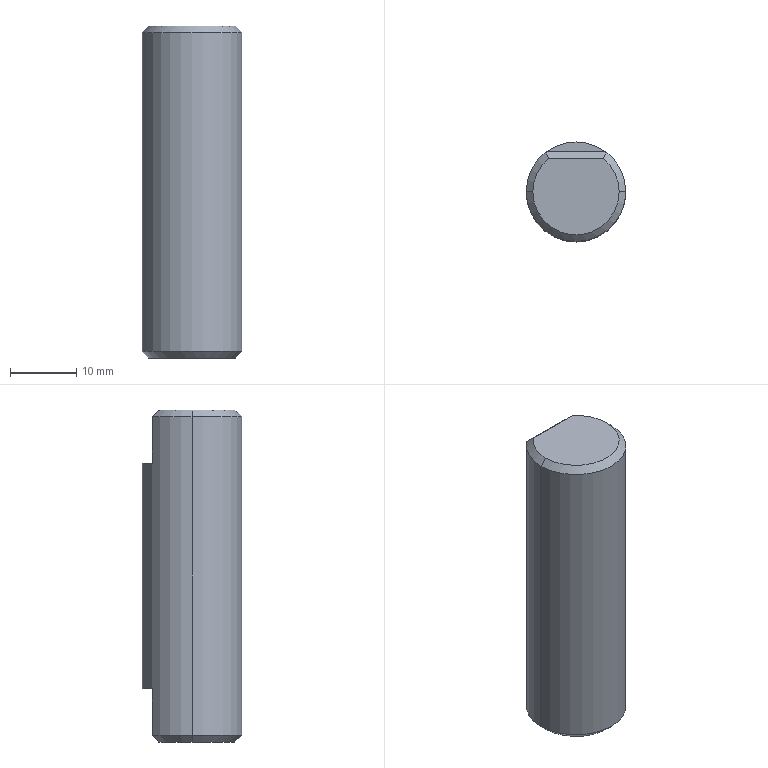Part | SolidWorks | features BaseBody 1 | 1 solid | 16 faces | box 15 x 15 x 50 mm | volume 8644 mm3 | plane 8 | cone 6 | cylinder 2 | commonest cylinder face diameters 15 x2
STEP:
#1=CARTESIAN_POINT('',(-6.5,0.,-25.));
#2=VERTEX_POINT('',#1);
#3=CARTESIAN_POINT('',(-4.153,5.,-25.));
#4=VERTEX_POINT('',#3);
#5=CARTESIAN_POINT('',(0.,0.,-25.));
#6=DIRECTION('',(0.,0.,-1.));
#7=DIRECTION('',(1.,0.,0.));
#8=AXIS2_PLACEMENT_3D('',#5,#6,#7);
#9=CIRCLE('',#8,6.5);
#10=EDGE_CURVE('',#2,#4,#9,.T.);
#11=ORIENTED_EDGE('',*,*,#10,.F.);
#12=CARTESIAN_POINT('',(-7.5,0.,-24.));
#13=VERTEX_POINT('',#12);
#14=CARTESIAN_POINT('',(-7.5,0.,-24.));
#15=DIRECTION('',(-0.7071,0.,0.7071));
#16=VECTOR('',#15,1000.);
#17=LINE('',#14,#16);
#18=EDGE_CURVE('',#2,#13,#17,.T.);
#19=ORIENTED_EDGE('',*,*,#18,.T.);
#20=CARTESIAN_POINT('',(-4.5,6.,-24.));
#21=VERTEX_POINT('',#20);
#22=CARTESIAN_POINT('',(0.,0.,-24.));
#23=DIRECTION('',(0.,0.,1.));
#24=DIRECTION('',(1.,0.,0.));
#25=AXIS2_PLACEMENT_3D('',#22,#23,#24);
#26=CIRCLE('',#25,7.5);
#27=EDGE_CURVE('',#21,#13,#26,.T.);
#28=ORIENTED_EDGE('',*,*,#27,.F.);
#29=CARTESIAN_POINT('',(-4.5,6.,-24.));
#30=CARTESIAN_POINT('',(-4.389,5.666,-24.334));
#31=CARTESIAN_POINT('',(-4.273,5.333,-24.667));
#32=CARTESIAN_POINT('',(-4.153,5.,-25.));
#33=B_SPLINE_CURVE_WITH_KNOTS('',3,(#29,#30,#31,#32),.UNSPECIFIED.,.F.,.F.,(4,4),(0.,0.001456),.UNSPECIFIED.);
#34=EDGE_CURVE('',#21,#4,#33,.T.);
#35=ORIENTED_EDGE('',*,*,#34,.T.);
#36=EDGE_LOOP('',(#11,#19,#28,#35));
#37=FACE_OUTER_BOUND('',#36,.T.);
#38=CARTESIAN_POINT('',(0.,0.,-24.));
#39=DIRECTION('',(0.,0.,1.));
#40=DIRECTION('',(1.,0.,0.));
#41=AXIS2_PLACEMENT_3D('',#38,#39,#40);
#42=CONICAL_SURFACE('',#41,7.5,0.7854);
#43=ADVANCED_FACE('',(#37),#42,.T.);
#44=ORIENTED_EDGE('',*,*,#18,.F.);
#45=CARTESIAN_POINT('',(6.5,0.,-25.));
#46=VERTEX_POINT('',#45);
#47=CARTESIAN_POINT('',(0.,0.,-25.));
#48=DIRECTION('',(0.,0.,-1.));
#49=DIRECTION('',(1.,0.,0.));
#50=AXIS2_PLACEMENT_3D('',#47,#48,#49);
#51=CIRCLE('',#50,6.5);
#52=EDGE_CURVE('',#46,#2,#51,.T.);
#53=ORIENTED_EDGE('',*,*,#52,.F.);
#54=CARTESIAN_POINT('',(7.5,0.,-24.));
#55=VERTEX_POINT('',#54);
#56=CARTESIAN_POINT('',(7.5,0.,-24.));
#57=DIRECTION('',(0.7071,0.,0.7071));
#58=VECTOR('',#57,1000.);
#59=LINE('',#56,#58);
#60=EDGE_CURVE('',#46,#55,#59,.T.);
#61=ORIENTED_EDGE('',*,*,#60,.T.);
#62=CARTESIAN_POINT('',(0.,0.,-24.));
#63=DIRECTION('',(0.,0.,1.));
#64=DIRECTION('',(1.,0.,0.));
#65=AXIS2_PLACEMENT_3D('',#62,#63,#64);
#66=CIRCLE('',#65,7.5);
#67=EDGE_CURVE('',#13,#55,#66,.T.);
#68=ORIENTED_EDGE('',*,*,#67,.F.);
#69=EDGE_LOOP('',(#44,#53,#61,#68));
#70=FACE_OUTER_BOUND('',#69,.T.);
#71=CARTESIAN_POINT('',(0.,0.,-24.));
#72=DIRECTION('',(0.,0.,1.));
#73=DIRECTION('',(1.,0.,0.));
#74=AXIS2_PLACEMENT_3D('',#71,#72,#73);
#75=CONICAL_SURFACE('',#74,7.5,0.7854);
#76=ADVANCED_FACE('',(#70),#75,.T.);
#77=CARTESIAN_POINT('',(6.5,0.,25.));
#78=VERTEX_POINT('',#77);
#79=CARTESIAN_POINT('',(4.153,5.,25.));
#80=VERTEX_POINT('',#79);
#81=CARTESIAN_POINT('',(0.,0.,25.));
#82=DIRECTION('',(0.,0.,1.));
#83=DIRECTION('',(1.,0.,0.));
#84=AXIS2_PLACEMENT_3D('',#81,#82,#83);
#85=CIRCLE('',#84,6.5);
#86=EDGE_CURVE('',#78,#80,#85,.T.);
#87=ORIENTED_EDGE('',*,*,#86,.F.);
#88=CARTESIAN_POINT('',(7.5,0.,24.));
#89=VERTEX_POINT('',#88);
#90=CARTESIAN_POINT('',(6.5,0.,25.));
#91=DIRECTION('',(0.7071,0.,-0.7071));
#92=VECTOR('',#91,1000.);
#93=LINE('',#90,#92);
#94=EDGE_CURVE('',#78,#89,#93,.T.);
#95=ORIENTED_EDGE('',*,*,#94,.T.);
#96=CARTESIAN_POINT('',(4.5,6.,24.));
#97=VERTEX_POINT('',#96);
#98=CARTESIAN_POINT('',(0.,0.,24.));
#99=DIRECTION('',(0.,0.,-1.));
#100=DIRECTION('',(1.,0.,0.));
#101=AXIS2_PLACEMENT_3D('',#98,#99,#100);
#102=CIRCLE('',#101,7.5);
#103=EDGE_CURVE('',#97,#89,#102,.T.);
#104=ORIENTED_EDGE('',*,*,#103,.F.);
#105=CARTESIAN_POINT('',(4.5,6.,24.));
#106=CARTESIAN_POINT('',(4.389,5.666,24.334));
#107=CARTESIAN_POINT('',(4.273,5.333,24.667));
#108=CARTESIAN_POINT('',(4.153,5.,25.));
#109=B_SPLINE_CURVE_WITH_KNOTS('',3,(#105,#106,#107,#108),.UNSPECIFIED.,.F.,.F.,(4,4),(0.,0.001456),.UNSPECIFIED.);
#110=EDGE_CURVE('',#97,#80,#109,.T.);
#111=ORIENTED_EDGE('',*,*,#110,.T.);
#112=EDGE_LOOP('',(#87,#95,#104,#111));
#113=FACE_OUTER_BOUND('',#112,.T.);
#114=CARTESIAN_POINT('',(0.,0.,25.));
#115=DIRECTION('',(0.,0.,-1.));
#116=DIRECTION('',(-1.,0.,0.));
#117=AXIS2_PLACEMENT_3D('',#114,#115,#116);
#118=CONICAL_SURFACE('',#117,6.5,0.7854);
#119=ADVANCED_FACE('',(#113),#118,.T.);
#120=ORIENTED_EDGE('',*,*,#94,.F.);
#121=CARTESIAN_POINT('',(-6.5,0.,25.));
#122=VERTEX_POINT('',#121);
#123=CARTESIAN_POINT('',(0.,0.,25.));
#124=DIRECTION('',(0.,0.,1.));
#125=DIRECTION('',(1.,0.,0.));
#126=AXIS2_PLACEMENT_3D('',#123,#124,#125);
#127=CIRCLE('',#126,6.5);
#128=EDGE_CURVE('',#122,#78,#127,.T.);
#129=ORIENTED_EDGE('',*,*,#128,.F.);
#130=CARTESIAN_POINT('',(-7.5,0.,24.));
#131=VERTEX_POINT('',#130);
#132=CARTESIAN_POINT('',(-6.5,0.,25.));
#133=DIRECTION('',(-0.7071,0.,-0.7071));
#134=VECTOR('',#133,1000.);
#135=LINE('',#132,#134);
#136=EDGE_CURVE('',#122,#131,#135,.T.);
#137=ORIENTED_EDGE('',*,*,#136,.T.);
#138=CARTESIAN_POINT('',(0.,0.,24.));
#139=DIRECTION('',(0.,0.,-1.));
#140=DIRECTION('',(1.,0.,0.));
#141=AXIS2_PLACEMENT_3D('',#138,#139,#140);
#142=CIRCLE('',#141,7.5);
#143=EDGE_CURVE('',#89,#131,#142,.T.);
#144=ORIENTED_EDGE('',*,*,#143,.F.);
#145=EDGE_LOOP('',(#120,#129,#137,#144));
#146=FACE_OUTER_BOUND('',#145,.T.);
#147=CARTESIAN_POINT('',(0.,0.,25.));
#148=DIRECTION('',(0.,0.,-1.));
#149=DIRECTION('',(-1.,0.,0.));
#150=AXIS2_PLACEMENT_3D('',#147,#148,#149);
#151=CONICAL_SURFACE('',#150,6.5,0.7854);
#152=ADVANCED_FACE('',(#146),#151,.T.);
#153=ORIENTED_EDGE('',*,*,#103,.T.);
#154=CARTESIAN_POINT('',(7.5,0.,25.));
#155=DIRECTION('',(0.,0.,-1.));
#156=VECTOR('',#155,1000.);
#157=LINE('',#154,#156);
#158=EDGE_CURVE('',#89,#55,#157,.T.);
#159=ORIENTED_EDGE('',*,*,#158,.T.);
#160=CARTESIAN_POINT('',(4.5,6.,-24.));
#161=VERTEX_POINT('',#160);
#162=CARTESIAN_POINT('',(0.,0.,-24.));
#163=DIRECTION('',(0.,0.,1.));
#164=DIRECTION('',(1.,0.,0.));
#165=AXIS2_PLACEMENT_3D('',#162,#163,#164);
#166=CIRCLE('',#165,7.5);
#167=EDGE_CURVE('',#55,#161,#166,.T.);
#168=ORIENTED_EDGE('',*,*,#167,.T.);
#169=CARTESIAN_POINT('',(4.5,6.,-17.));
#170=VERTEX_POINT('',#169);
#171=CARTESIAN_POINT('',(4.5,6.,-17.));
#172=DIRECTION('',(0.,0.,-1.));
#173=VECTOR('',#172,1000.);
#174=LINE('',#171,#173);
#175=EDGE_CURVE('',#170,#161,#174,.T.);
#176=ORIENTED_EDGE('',*,*,#175,.F.);
#177=CARTESIAN_POINT('',(-4.5,6.,-17.));
#178=VERTEX_POINT('',#177);
#179=CARTESIAN_POINT('',(0.,0.,-17.));
#180=DIRECTION('',(0.,0.,1.));
#181=DIRECTION('',(1.,0.,0.));
#182=AXIS2_PLACEMENT_3D('',#179,#180,#181);
#183=CIRCLE('',#182,7.5);
#184=EDGE_CURVE('',#170,#178,#183,.T.);
#185=ORIENTED_EDGE('',*,*,#184,.T.);
#186=CARTESIAN_POINT('',(-4.5,6.,-17.));
#187=DIRECTION('',(0.,0.,-1.));
#188=VECTOR('',#187,1000.);
#189=LINE('',#186,#188);
#190=EDGE_CURVE('',#178,#21,#189,.T.);
#191=ORIENTED_EDGE('',*,*,#190,.T.);
#192=ORIENTED_EDGE('',*,*,#27,.T.);
#193=CARTESIAN_POINT('',(-7.5,0.,25.));
#194=DIRECTION('',(0.,0.,-1.));
#195=VECTOR('',#194,1000.);
#196=LINE('',#193,#195);
#197=EDGE_CURVE('',#131,#13,#196,.T.);
#198=ORIENTED_EDGE('',*,*,#197,.F.);
#199=CARTESIAN_POINT('',(-4.5,6.,24.));
#200=VERTEX_POINT('',#199);
#201=CARTESIAN_POINT('',(0.,0.,24.));
#202=DIRECTION('',(0.,0.,-1.));
#203=DIRECTION('',(1.,0.,0.));
#204=AXIS2_PLACEMENT_3D('',#201,#202,#203);
#205=CIRCLE('',#204,7.5);
#206=EDGE_CURVE('',#131,#200,#205,.T.);
#207=ORIENTED_EDGE('',*,*,#206,.T.);
#208=CARTESIAN_POINT('',(-4.5,6.,17.));
#209=VERTEX_POINT('',#208);
#210=CARTESIAN_POINT('',(-4.5,6.,17.));
#211=DIRECTION('',(0.,0.,1.));
#212=VECTOR('',#211,1000.);
#213=LINE('',#210,#212);
#214=EDGE_CURVE('',#209,#200,#213,.T.);
#215=ORIENTED_EDGE('',*,*,#214,.F.);
#216=CARTESIAN_POINT('',(4.5,6.,17.));
#217=VERTEX_POINT('',#216);
#218=CARTESIAN_POINT('',(0.,0.,17.));
#219=DIRECTION('',(0.,0.,1.));
#220=DIRECTION('',(1.,0.,0.));
#221=AXIS2_PLACEMENT_3D('',#218,#219,#220);
#222=CIRCLE('',#221,7.5);
#223=EDGE_CURVE('',#217,#209,#222,.T.);
#224=ORIENTED_EDGE('',*,*,#223,.F.);
#225=CARTESIAN_POINT('',(4.5,6.,17.));
#226=DIRECTION('',(0.,0.,1.));
#227=VECTOR('',#226,1000.);
#228=LINE('',#225,#227);
#229=EDGE_CURVE('',#217,#97,#228,.T.);
#230=ORIENTED_EDGE('',*,*,#229,.T.);
#231=EDGE_LOOP('',(#153,#159,#168,#176,#185,#191,#192,#198,#207,#215,#224,#230));
#232=FACE_OUTER_BOUND('',#231,.T.);
#233=CARTESIAN_POINT('',(0.,0.,25.));
#234=DIRECTION('',(0.,0.,-1.));
#235=DIRECTION('',(-1.,0.,0.));
#236=AXIS2_PLACEMENT_3D('',#233,#234,#235);
#237=CYLINDRICAL_SURFACE('',#236,7.5);
#238=ADVANCED_FACE('',(#232),#237,.T.);
#239=ORIENTED_EDGE('',*,*,#158,.F.);
#240=ORIENTED_EDGE('',*,*,#143,.T.);
#241=ORIENTED_EDGE('',*,*,#197,.T.);
#242=ORIENTED_EDGE('',*,*,#67,.T.);
#243=EDGE_LOOP('',(#239,#240,#241,#242));
#244=FACE_OUTER_BOUND('',#243,.T.);
#245=CARTESIAN_POINT('',(0.,0.,25.));
#246=DIRECTION('',(0.,0.,-1.));
#247=DIRECTION('',(-1.,0.,0.));
#248=AXIS2_PLACEMENT_3D('',#245,#246,#247);
#249=CYLINDRICAL_SURFACE('',#248,7.5);
#250=ADVANCED_FACE('',(#244),#249,.T.);
#251=CARTESIAN_POINT('',(4.153,5.,-25.));
#252=VERTEX_POINT('',#251);
#253=CARTESIAN_POINT('',(4.5,5.,-25.));
#254=DIRECTION('',(1.,0.,0.));
#255=VECTOR('',#254,1000.);
#256=LINE('',#253,#255);
#257=EDGE_CURVE('',#4,#252,#256,.T.);
#258=ORIENTED_EDGE('',*,*,#257,.T.);
#259=CARTESIAN_POINT('',(0.,0.,-25.));
#260=DIRECTION('',(0.,0.,-1.));
#261=DIRECTION('',(1.,0.,0.));
#262=AXIS2_PLACEMENT_3D('',#259,#260,#261);
#263=CIRCLE('',#262,6.5);
#264=EDGE_CURVE('',#252,#46,#263,.T.);
#265=ORIENTED_EDGE('',*,*,#264,.T.);
#266=ORIENTED_EDGE('',*,*,#52,.T.);
#267=ORIENTED_EDGE('',*,*,#10,.T.);
#268=EDGE_LOOP('',(#258,#265,#266,#267));
#269=FACE_OUTER_BOUND('',#268,.T.);
#270=CARTESIAN_POINT('',(0.,0.,-25.));
#271=DIRECTION('',(0.,0.,1.));
#272=DIRECTION('',(1.,0.,0.));
#273=AXIS2_PLACEMENT_3D('',#270,#271,#272);
#274=PLANE('',#273);
#275=ADVANCED_FACE('',(#269),#274,.F.);
#276=CARTESIAN_POINT('',(-4.153,5.,25.));
#277=VERTEX_POINT('',#276);
#278=CARTESIAN_POINT('',(-4.5,5.,25.));
#279=DIRECTION('',(-1.,0.,0.));
#280=VECTOR('',#279,1000.);
#281=LINE('',#278,#280);
#282=EDGE_CURVE('',#80,#277,#281,.T.);
#283=ORIENTED_EDGE('',*,*,#282,.T.);
#284=CARTESIAN_POINT('',(0.,0.,25.));
#285=DIRECTION('',(0.,0.,1.));
#286=DIRECTION('',(1.,0.,0.));
#287=AXIS2_PLACEMENT_3D('',#284,#285,#286);
#288=CIRCLE('',#287,6.5);
#289=EDGE_CURVE('',#277,#122,#288,.T.);
#290=ORIENTED_EDGE('',*,*,#289,.T.);
#291=ORIENTED_EDGE('',*,*,#128,.T.);
#292=ORIENTED_EDGE('',*,*,#86,.T.);
#293=EDGE_LOOP('',(#283,#290,#291,#292));
#294=FACE_OUTER_BOUND('',#293,.T.);
#295=CARTESIAN_POINT('',(0.,0.,25.));
#296=DIRECTION('',(0.,0.,1.));
#297=DIRECTION('',(1.,0.,0.));
#298=AXIS2_PLACEMENT_3D('',#295,#296,#297);
#299=PLANE('',#298);
#300=ADVANCED_FACE('',(#294),#299,.T.);
#301=ORIENTED_EDGE('',*,*,#214,.T.);
#302=CARTESIAN_POINT('',(4.5,6.,24.));
#303=DIRECTION('',(1.,0.,0.));
#304=VECTOR('',#303,1000.);
#305=LINE('',#302,#304);
#306=EDGE_CURVE('',#200,#97,#305,.T.);
#307=ORIENTED_EDGE('',*,*,#306,.T.);
#308=ORIENTED_EDGE('',*,*,#229,.F.);
#309=CARTESIAN_POINT('',(-4.5,6.,17.));
#310=DIRECTION('',(1.,0.,0.));
#311=VECTOR('',#310,1000.);
#312=LINE('',#309,#311);
#313=EDGE_CURVE('',#209,#217,#312,.T.);
#314=ORIENTED_EDGE('',*,*,#313,.F.);
#315=EDGE_LOOP('',(#301,#307,#308,#314));
#316=FACE_OUTER_BOUND('',#315,.T.);
#317=CARTESIAN_POINT('',(-4.5,6.,17.));
#318=DIRECTION('',(0.,-1.,0.));
#319=DIRECTION('',(0.,0.,-1.));
#320=AXIS2_PLACEMENT_3D('',#317,#318,#319);
#321=PLANE('',#320);
#322=ADVANCED_FACE('',(#316),#321,.F.);
#323=ORIENTED_EDGE('',*,*,#223,.T.);
#324=ORIENTED_EDGE('',*,*,#313,.T.);
#325=EDGE_LOOP('',(#323,#324));
#326=FACE_OUTER_BOUND('',#325,.T.);
#327=CARTESIAN_POINT('',(0.,0.,17.));
#328=DIRECTION('',(0.,0.,1.));
#329=DIRECTION('',(1.,0.,0.));
#330=AXIS2_PLACEMENT_3D('',#327,#328,#329);
#331=PLANE('',#330);
#332=ADVANCED_FACE('',(#326),#331,.T.);
#333=ORIENTED_EDGE('',*,*,#175,.T.);
#334=CARTESIAN_POINT('',(-4.5,6.,-24.));
#335=DIRECTION('',(-1.,0.,0.));
#336=VECTOR('',#335,1000.);
#337=LINE('',#334,#336);
#338=EDGE_CURVE('',#161,#21,#337,.T.);
#339=ORIENTED_EDGE('',*,*,#338,.T.);
#340=ORIENTED_EDGE('',*,*,#190,.F.);
#341=CARTESIAN_POINT('',(-4.5,6.,-17.));
#342=DIRECTION('',(1.,0.,0.));
#343=VECTOR('',#342,1000.);
#344=LINE('',#341,#343);
#345=EDGE_CURVE('',#178,#170,#344,.T.);
#346=ORIENTED_EDGE('',*,*,#345,.T.);
#347=EDGE_LOOP('',(#333,#339,#340,#346));
#348=FACE_OUTER_BOUND('',#347,.T.);
#349=CARTESIAN_POINT('',(-4.5,6.,-17.));
#350=DIRECTION('',(0.,1.,0.));
#351=DIRECTION('',(0.,0.,1.));
#352=AXIS2_PLACEMENT_3D('',#349,#350,#351);
#353=PLANE('',#352);
#354=ADVANCED_FACE('',(#348),#353,.T.);
#355=ORIENTED_EDGE('',*,*,#184,.F.);
#356=ORIENTED_EDGE('',*,*,#345,.F.);
#357=EDGE_LOOP('',(#355,#356));
#358=FACE_OUTER_BOUND('',#357,.T.);
#359=CARTESIAN_POINT('',(0.,0.,-17.));
#360=DIRECTION('',(0.,0.,-1.));
#361=DIRECTION('',(1.,0.,0.));
#362=AXIS2_PLACEMENT_3D('',#359,#360,#361);
#363=PLANE('',#362);
#364=ADVANCED_FACE('',(#358),#363,.T.);
#365=ORIENTED_EDGE('',*,*,#110,.F.);
#366=ORIENTED_EDGE('',*,*,#306,.F.);
#367=CARTESIAN_POINT('',(-4.153,5.,25.));
#368=CARTESIAN_POINT('',(-4.273,5.333,24.667));
#369=CARTESIAN_POINT('',(-4.389,5.666,24.334));
#370=CARTESIAN_POINT('',(-4.5,6.,24.));
#371=B_SPLINE_CURVE_WITH_KNOTS('',3,(#367,#368,#369,#370),.UNSPECIFIED.,.F.,.F.,(4,4),(0.,0.001456),.UNSPECIFIED.);
#372=EDGE_CURVE('',#277,#200,#371,.T.);
#373=ORIENTED_EDGE('',*,*,#372,.F.);
#374=ORIENTED_EDGE('',*,*,#282,.F.);
#375=EDGE_LOOP('',(#365,#366,#373,#374));
#376=FACE_OUTER_BOUND('',#375,.T.);
#377=CARTESIAN_POINT('',(-4.5,6.,24.));
#378=DIRECTION('',(0.,0.7071,0.7071));
#379=DIRECTION('',(0.,-0.7071,0.7071));
#380=AXIS2_PLACEMENT_3D('',#377,#378,#379);
#381=PLANE('',#380);
#382=ADVANCED_FACE('',(#376),#381,.T.);
#383=ORIENTED_EDGE('',*,*,#136,.F.);
#384=ORIENTED_EDGE('',*,*,#289,.F.);
#385=ORIENTED_EDGE('',*,*,#372,.T.);
#386=ORIENTED_EDGE('',*,*,#206,.F.);
#387=EDGE_LOOP('',(#383,#384,#385,#386));
#388=FACE_OUTER_BOUND('',#387,.T.);
#389=CARTESIAN_POINT('',(0.,0.,25.));
#390=DIRECTION('',(0.,0.,-1.));
#391=DIRECTION('',(-1.,0.,0.));
#392=AXIS2_PLACEMENT_3D('',#389,#390,#391);
#393=CONICAL_SURFACE('',#392,6.5,0.7854);
#394=ADVANCED_FACE('',(#388),#393,.T.);
#395=CARTESIAN_POINT('',(4.153,5.,-25.));
#396=CARTESIAN_POINT('',(4.273,5.333,-24.667));
#397=CARTESIAN_POINT('',(4.389,5.666,-24.334));
#398=CARTESIAN_POINT('',(4.5,6.,-24.));
#399=B_SPLINE_CURVE_WITH_KNOTS('',3,(#395,#396,#397,#398),.UNSPECIFIED.,.F.,.F.,(4,4),(0.,0.001456),.UNSPECIFIED.);
#400=EDGE_CURVE('',#252,#161,#399,.T.);
#401=ORIENTED_EDGE('',*,*,#400,.F.);
#402=ORIENTED_EDGE('',*,*,#257,.F.);
#403=ORIENTED_EDGE('',*,*,#34,.F.);
#404=ORIENTED_EDGE('',*,*,#338,.F.);
#405=EDGE_LOOP('',(#401,#402,#403,#404));
#406=FACE_OUTER_BOUND('',#405,.T.);
#407=CARTESIAN_POINT('',(0.,5.,-25.));
#408=DIRECTION('',(0.,0.7071,-0.7071));
#409=DIRECTION('',(0.,0.7071,0.7071));
#410=AXIS2_PLACEMENT_3D('',#407,#408,#409);
#411=PLANE('',#410);
#412=ADVANCED_FACE('',(#406),#411,.T.);
#413=ORIENTED_EDGE('',*,*,#60,.F.);
#414=ORIENTED_EDGE('',*,*,#264,.F.);
#415=ORIENTED_EDGE('',*,*,#400,.T.);
#416=ORIENTED_EDGE('',*,*,#167,.F.);
#417=EDGE_LOOP('',(#413,#414,#415,#416));
#418=FACE_OUTER_BOUND('',#417,.T.);
#419=CARTESIAN_POINT('',(0.,0.,-24.));
#420=DIRECTION('',(0.,0.,1.));
#421=DIRECTION('',(1.,0.,0.));
#422=AXIS2_PLACEMENT_3D('',#419,#420,#421);
#423=CONICAL_SURFACE('',#422,7.5,0.7854);
#424=ADVANCED_FACE('',(#418),#423,.T.);
#425=CLOSED_SHELL('',(#43,#76,#119,#152,#238,#250,#275,#300,#322,#332,#354,#364,#382,#394,#412,#424));
#426=MANIFOLD_SOLID_BREP('',#425);
#427=CARTESIAN_POINT('',(0.,0.,0.));
#428=DIRECTION('',(0.,0.,1.));
#429=DIRECTION('',(1.,0.,0.));
#430=AXIS2_PLACEMENT_3D('',#427,#428,#429);
#431=(LENGTH_UNIT()NAMED_UNIT(*)SI_UNIT(.MILLI.,.METRE.));
#432=UNCERTAINTY_MEASURE_WITH_UNIT(LENGTH_MEASURE(0.00001),#431,'','');
#433=(NAMED_UNIT(*)PLANE_ANGLE_UNIT()SI_UNIT($,.RADIAN.));
#434=(NAMED_UNIT(*)SI_UNIT($,.STERADIAN.)SOLID_ANGLE_UNIT());
#435=(GEOMETRIC_REPRESENTATION_CONTEXT(3)GLOBAL_UNCERTAINTY_ASSIGNED_CONTEXT((#432))GLOBAL_UNIT_ASSIGNED_CONTEXT((#431,#433,#434))REPRESENTATION_CONTEXT('',''));
#436=ADVANCED_BREP_SHAPE_REPRESENTATION('',(#426,#430),#435);